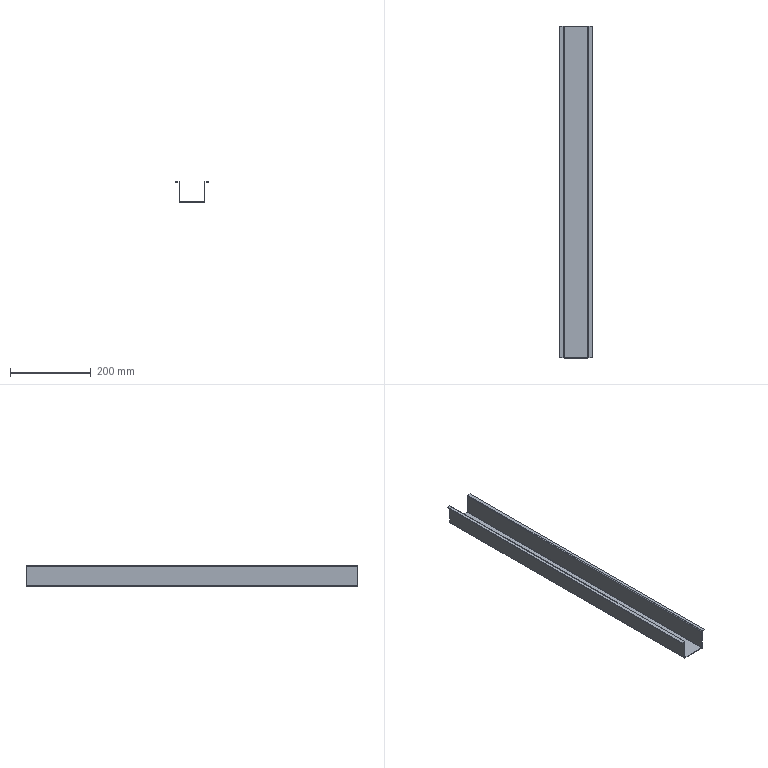Part | SolidWorks | features BaseBody 1 | 1 solid | 38 faces | box 80 x 820 x 51.5 mm | volume 218760 mm3 | plane 30 | cylinder 8 | commonest cylinder face diameters 1 x4 4 x4
STEP:
#1=CARTESIAN_POINT('',(40.,-410.,48.5));
#2=VERTEX_POINT('',#1);
#3=CARTESIAN_POINT('',(40.,410.,48.5));
#4=VERTEX_POINT('',#3);
#5=CARTESIAN_POINT('',(40.,410.,48.5));
#6=DIRECTION('',(0.,1.,0.));
#7=VECTOR('',#6,1000.);
#8=LINE('',#5,#7);
#9=EDGE_CURVE('',#2,#4,#8,.T.);
#10=ORIENTED_EDGE('',*,*,#9,.T.);
#11=CARTESIAN_POINT('',(40.,410.,50.));
#12=VERTEX_POINT('',#11);
#13=CARTESIAN_POINT('',(40.,410.,50.));
#14=DIRECTION('',(0.,0.,-1.));
#15=VECTOR('',#14,1000.);
#16=LINE('',#13,#15);
#17=EDGE_CURVE('',#12,#4,#16,.T.);
#18=ORIENTED_EDGE('',*,*,#17,.F.);
#19=CARTESIAN_POINT('',(40.,-410.,50.));
#20=VERTEX_POINT('',#19);
#21=CARTESIAN_POINT('',(40.,410.,50.));
#22=DIRECTION('',(0.,1.,0.));
#23=VECTOR('',#22,1000.);
#24=LINE('',#21,#23);
#25=EDGE_CURVE('',#20,#12,#24,.T.);
#26=ORIENTED_EDGE('',*,*,#25,.F.);
#27=CARTESIAN_POINT('',(40.,-410.,50.));
#28=DIRECTION('',(0.,0.,-1.));
#29=VECTOR('',#28,1000.);
#30=LINE('',#27,#29);
#31=EDGE_CURVE('',#20,#2,#30,.T.);
#32=ORIENTED_EDGE('',*,*,#31,.T.);
#33=EDGE_LOOP('',(#10,#18,#26,#32));
#34=FACE_OUTER_BOUND('',#33,.T.);
#35=CARTESIAN_POINT('',(40.,410.,50.));
#36=DIRECTION('',(-1.,0.,0.));
#37=DIRECTION('',(0.,1.,0.));
#38=AXIS2_PLACEMENT_3D('',#35,#36,#37);
#39=PLANE('',#38);
#40=ADVANCED_FACE('',(#34),#39,.F.);
#41=CARTESIAN_POINT('',(32.,-410.,48.5));
#42=VERTEX_POINT('',#41);
#43=CARTESIAN_POINT('',(40.,-410.,48.5));
#44=DIRECTION('',(1.,0.,0.));
#45=VECTOR('',#44,1000.);
#46=LINE('',#43,#45);
#47=EDGE_CURVE('',#42,#2,#46,.T.);
#48=ORIENTED_EDGE('',*,*,#47,.F.);
#49=CARTESIAN_POINT('',(32.,410.,48.5));
#50=VERTEX_POINT('',#49);
#51=CARTESIAN_POINT('',(32.,410.,48.5));
#52=DIRECTION('',(0.,-1.,0.));
#53=VECTOR('',#52,1000.);
#54=LINE('',#51,#53);
#55=EDGE_CURVE('',#50,#42,#54,.T.);
#56=ORIENTED_EDGE('',*,*,#55,.F.);
#57=CARTESIAN_POINT('',(31.5,410.,48.5));
#58=DIRECTION('',(-1.,0.,0.));
#59=VECTOR('',#58,1000.);
#60=LINE('',#57,#59);
#61=EDGE_CURVE('',#4,#50,#60,.T.);
#62=ORIENTED_EDGE('',*,*,#61,.F.);
#63=ORIENTED_EDGE('',*,*,#9,.F.);
#64=EDGE_LOOP('',(#48,#56,#62,#63));
#65=FACE_OUTER_BOUND('',#64,.T.);
#66=CARTESIAN_POINT('',(0.,0.,48.5));
#67=DIRECTION('',(0.,0.,-1.));
#68=DIRECTION('',(0.,-1.,0.));
#69=AXIS2_PLACEMENT_3D('',#66,#67,#68);
#70=PLANE('',#69);
#71=ADVANCED_FACE('',(#65),#70,.T.);
#72=CARTESIAN_POINT('',(32.,-410.,50.));
#73=VERTEX_POINT('',#72);
#74=CARTESIAN_POINT('',(32.,410.,50.));
#75=VERTEX_POINT('',#74);
#76=CARTESIAN_POINT('',(32.,0.,50.));
#77=DIRECTION('',(0.,1.,0.));
#78=VECTOR('',#77,1000.);
#79=LINE('',#76,#78);
#80=EDGE_CURVE('',#73,#75,#79,.T.);
#81=ORIENTED_EDGE('',*,*,#80,.F.);
#82=CARTESIAN_POINT('',(40.,-410.,50.));
#83=DIRECTION('',(1.,0.,0.));
#84=VECTOR('',#83,1000.);
#85=LINE('',#82,#84);
#86=EDGE_CURVE('',#73,#20,#85,.T.);
#87=ORIENTED_EDGE('',*,*,#86,.T.);
#88=ORIENTED_EDGE('',*,*,#25,.T.);
#89=CARTESIAN_POINT('',(31.5,410.,50.));
#90=DIRECTION('',(-1.,0.,0.));
#91=VECTOR('',#90,1000.);
#92=LINE('',#89,#91);
#93=EDGE_CURVE('',#12,#75,#92,.T.);
#94=ORIENTED_EDGE('',*,*,#93,.T.);
#95=EDGE_LOOP('',(#81,#87,#88,#94));
#96=FACE_OUTER_BOUND('',#95,.T.);
#97=CARTESIAN_POINT('',(0.,0.,50.));
#98=DIRECTION('',(0.,0.,-1.));
#99=DIRECTION('',(0.,-1.,0.));
#100=AXIS2_PLACEMENT_3D('',#97,#98,#99);
#101=PLANE('',#100);
#102=ADVANCED_FACE('',(#96),#101,.F.);
#103=CARTESIAN_POINT('',(32.,-410.,48.5));
#104=DIRECTION('',(0.,0.,1.));
#105=VECTOR('',#104,1000.);
#106=LINE('',#103,#105);
#107=EDGE_CURVE('',#42,#73,#106,.T.);
#108=ORIENTED_EDGE('',*,*,#107,.F.);
#109=ORIENTED_EDGE('',*,*,#47,.T.);
#110=ORIENTED_EDGE('',*,*,#31,.F.);
#111=ORIENTED_EDGE('',*,*,#86,.F.);
#112=EDGE_LOOP('',(#108,#109,#110,#111));
#113=FACE_OUTER_BOUND('',#112,.T.);
#114=CARTESIAN_POINT('',(40.,-410.,50.));
#115=DIRECTION('',(0.,1.,0.));
#116=DIRECTION('',(0.,0.,-1.));
#117=AXIS2_PLACEMENT_3D('',#114,#115,#116);
#118=PLANE('',#117);
#119=ADVANCED_FACE('',(#113),#118,.F.);
#120=CARTESIAN_POINT('',(32.,410.,48.5));
#121=DIRECTION('',(0.,0.,1.));
#122=VECTOR('',#121,1000.);
#123=LINE('',#120,#122);
#124=EDGE_CURVE('',#50,#75,#123,.T.);
#125=ORIENTED_EDGE('',*,*,#124,.T.);
#126=ORIENTED_EDGE('',*,*,#93,.F.);
#127=ORIENTED_EDGE('',*,*,#17,.T.);
#128=ORIENTED_EDGE('',*,*,#61,.T.);
#129=EDGE_LOOP('',(#125,#126,#127,#128));
#130=FACE_OUTER_BOUND('',#129,.T.);
#131=CARTESIAN_POINT('',(31.5,410.,50.));
#132=DIRECTION('',(0.,-1.,0.));
#133=DIRECTION('',(-1.,0.,0.));
#134=AXIS2_PLACEMENT_3D('',#131,#132,#133);
#135=PLANE('',#134);
#136=ADVANCED_FACE('',(#130),#135,.F.);
#137=CARTESIAN_POINT('',(31.5,-410.,48.));
#138=VERTEX_POINT('',#137);
#139=CARTESIAN_POINT('',(31.5,410.,48.));
#140=VERTEX_POINT('',#139);
#141=CARTESIAN_POINT('',(31.5,-410.,48.));
#142=DIRECTION('',(0.,1.,0.));
#143=VECTOR('',#142,1000.);
#144=LINE('',#141,#143);
#145=EDGE_CURVE('',#138,#140,#144,.T.);
#146=ORIENTED_EDGE('',*,*,#145,.T.);
#147=CARTESIAN_POINT('',(32.,410.,48.));
#148=DIRECTION('',(0.,1.,0.));
#149=DIRECTION('',(0.,0.,-1.));
#150=AXIS2_PLACEMENT_3D('',#147,#148,#149);
#151=CIRCLE('',#150,0.5);
#152=EDGE_CURVE('',#140,#50,#151,.T.);
#153=ORIENTED_EDGE('',*,*,#152,.T.);
#154=ORIENTED_EDGE('',*,*,#55,.T.);
#155=CARTESIAN_POINT('',(32.,-410.,48.));
#156=DIRECTION('',(0.,-1.,0.));
#157=DIRECTION('',(0.,0.,-1.));
#158=AXIS2_PLACEMENT_3D('',#155,#156,#157);
#159=CIRCLE('',#158,0.5);
#160=EDGE_CURVE('',#42,#138,#159,.T.);
#161=ORIENTED_EDGE('',*,*,#160,.T.);
#162=EDGE_LOOP('',(#146,#153,#154,#161));
#163=FACE_OUTER_BOUND('',#162,.T.);
#164=CARTESIAN_POINT('',(32.,-410.,48.));
#165=DIRECTION('',(0.,-1.,0.));
#166=DIRECTION('',(0.,0.,1.));
#167=AXIS2_PLACEMENT_3D('',#164,#165,#166);
#168=CYLINDRICAL_SURFACE('',#167,0.5);
#169=ADVANCED_FACE('',(#163),#168,.F.);
#170=CARTESIAN_POINT('',(30.,-410.,48.));
#171=VERTEX_POINT('',#170);
#172=CARTESIAN_POINT('',(30.,410.,48.));
#173=VERTEX_POINT('',#172);
#174=CARTESIAN_POINT('',(30.,-410.,48.));
#175=DIRECTION('',(0.,1.,0.));
#176=VECTOR('',#175,1000.);
#177=LINE('',#174,#176);
#178=EDGE_CURVE('',#171,#173,#177,.T.);
#179=ORIENTED_EDGE('',*,*,#178,.F.);
#180=CARTESIAN_POINT('',(32.,-410.,48.));
#181=DIRECTION('',(0.,-1.,0.));
#182=DIRECTION('',(0.,0.,-1.));
#183=AXIS2_PLACEMENT_3D('',#180,#181,#182);
#184=CIRCLE('',#183,2.);
#185=EDGE_CURVE('',#73,#171,#184,.T.);
#186=ORIENTED_EDGE('',*,*,#185,.F.);
#187=ORIENTED_EDGE('',*,*,#80,.T.);
#188=CARTESIAN_POINT('',(32.,410.,48.));
#189=DIRECTION('',(0.,1.,0.));
#190=DIRECTION('',(0.,0.,-1.));
#191=AXIS2_PLACEMENT_3D('',#188,#189,#190);
#192=CIRCLE('',#191,2.);
#193=EDGE_CURVE('',#173,#75,#192,.T.);
#194=ORIENTED_EDGE('',*,*,#193,.F.);
#195=EDGE_LOOP('',(#179,#186,#187,#194));
#196=FACE_OUTER_BOUND('',#195,.T.);
#197=CARTESIAN_POINT('',(32.,-410.,48.));
#198=DIRECTION('',(0.,-1.,0.));
#199=DIRECTION('',(0.,0.,1.));
#200=AXIS2_PLACEMENT_3D('',#197,#198,#199);
#201=CYLINDRICAL_SURFACE('',#200,2.);
#202=ADVANCED_FACE('',(#196),#201,.T.);
#203=ORIENTED_EDGE('',*,*,#160,.F.);
#204=ORIENTED_EDGE('',*,*,#107,.T.);
#205=ORIENTED_EDGE('',*,*,#185,.T.);
#206=CARTESIAN_POINT('',(31.5,-410.,48.));
#207=DIRECTION('',(-1.,0.,0.));
#208=VECTOR('',#207,1000.);
#209=LINE('',#206,#208);
#210=EDGE_CURVE('',#138,#171,#209,.T.);
#211=ORIENTED_EDGE('',*,*,#210,.F.);
#212=EDGE_LOOP('',(#203,#204,#205,#211));
#213=FACE_OUTER_BOUND('',#212,.T.);
#214=CARTESIAN_POINT('',(32.,-410.,48.));
#215=DIRECTION('',(0.,1.,0.));
#216=DIRECTION('',(1.,0.,0.));
#217=AXIS2_PLACEMENT_3D('',#214,#215,#216);
#218=PLANE('',#217);
#219=ADVANCED_FACE('',(#213),#218,.F.);
#220=ORIENTED_EDGE('',*,*,#124,.F.);
#221=ORIENTED_EDGE('',*,*,#152,.F.);
#222=CARTESIAN_POINT('',(31.5,410.,48.));
#223=DIRECTION('',(-1.,0.,0.));
#224=VECTOR('',#223,1000.);
#225=LINE('',#222,#224);
#226=EDGE_CURVE('',#140,#173,#225,.T.);
#227=ORIENTED_EDGE('',*,*,#226,.T.);
#228=ORIENTED_EDGE('',*,*,#193,.T.);
#229=EDGE_LOOP('',(#220,#221,#227,#228));
#230=FACE_OUTER_BOUND('',#229,.T.);
#231=CARTESIAN_POINT('',(32.,410.,48.));
#232=DIRECTION('',(0.,1.,0.));
#233=DIRECTION('',(1.,0.,0.));
#234=AXIS2_PLACEMENT_3D('',#231,#232,#233);
#235=PLANE('',#234);
#236=ADVANCED_FACE('',(#230),#235,.T.);
#237=CARTESIAN_POINT('',(-40.,410.,48.5));
#238=VERTEX_POINT('',#237);
#239=CARTESIAN_POINT('',(-40.,-410.,48.5));
#240=VERTEX_POINT('',#239);
#241=CARTESIAN_POINT('',(-40.,-410.,48.5));
#242=DIRECTION('',(0.,-1.,0.));
#243=VECTOR('',#242,1000.);
#244=LINE('',#241,#243);
#245=EDGE_CURVE('',#238,#240,#244,.T.);
#246=ORIENTED_EDGE('',*,*,#245,.T.);
#247=CARTESIAN_POINT('',(-40.,-410.,50.));
#248=VERTEX_POINT('',#247);
#249=CARTESIAN_POINT('',(-40.,-410.,50.));
#250=DIRECTION('',(0.,0.,-1.));
#251=VECTOR('',#250,1000.);
#252=LINE('',#249,#251);
#253=EDGE_CURVE('',#248,#240,#252,.T.);
#254=ORIENTED_EDGE('',*,*,#253,.F.);
#255=CARTESIAN_POINT('',(-40.,410.,50.));
#256=VERTEX_POINT('',#255);
#257=CARTESIAN_POINT('',(-40.,-410.,50.));
#258=DIRECTION('',(0.,-1.,0.));
#259=VECTOR('',#258,1000.);
#260=LINE('',#257,#259);
#261=EDGE_CURVE('',#256,#248,#260,.T.);
#262=ORIENTED_EDGE('',*,*,#261,.F.);
#263=CARTESIAN_POINT('',(-40.,410.,50.));
#264=DIRECTION('',(0.,0.,-1.));
#265=VECTOR('',#264,1000.);
#266=LINE('',#263,#265);
#267=EDGE_CURVE('',#256,#238,#266,.T.);
#268=ORIENTED_EDGE('',*,*,#267,.T.);
#269=EDGE_LOOP('',(#246,#254,#262,#268));
#270=FACE_OUTER_BOUND('',#269,.T.);
#271=CARTESIAN_POINT('',(-40.,-410.,50.));
#272=DIRECTION('',(1.,0.,0.));
#273=DIRECTION('',(0.,1.,0.));
#274=AXIS2_PLACEMENT_3D('',#271,#272,#273);
#275=PLANE('',#274);
#276=ADVANCED_FACE('',(#270),#275,.F.);
#277=CARTESIAN_POINT('',(-32.,410.,48.5));
#278=VERTEX_POINT('',#277);
#279=CARTESIAN_POINT('',(-40.,410.,48.5));
#280=DIRECTION('',(-1.,0.,0.));
#281=VECTOR('',#280,1000.);
#282=LINE('',#279,#281);
#283=EDGE_CURVE('',#278,#238,#282,.T.);
#284=ORIENTED_EDGE('',*,*,#283,.F.);
#285=CARTESIAN_POINT('',(-32.,-410.,48.5));
#286=VERTEX_POINT('',#285);
#287=CARTESIAN_POINT('',(-32.,-410.,48.5));
#288=DIRECTION('',(0.,1.,0.));
#289=VECTOR('',#288,1000.);
#290=LINE('',#287,#289);
#291=EDGE_CURVE('',#286,#278,#290,.T.);
#292=ORIENTED_EDGE('',*,*,#291,.F.);
#293=CARTESIAN_POINT('',(-31.5,-410.,48.5));
#294=DIRECTION('',(1.,0.,0.));
#295=VECTOR('',#294,1000.);
#296=LINE('',#293,#295);
#297=EDGE_CURVE('',#240,#286,#296,.T.);
#298=ORIENTED_EDGE('',*,*,#297,.F.);
#299=ORIENTED_EDGE('',*,*,#245,.F.);
#300=EDGE_LOOP('',(#284,#292,#298,#299));
#301=FACE_OUTER_BOUND('',#300,.T.);
#302=CARTESIAN_POINT('',(0.,0.,48.5));
#303=DIRECTION('',(0.,0.,-1.));
#304=DIRECTION('',(0.,-1.,0.));
#305=AXIS2_PLACEMENT_3D('',#302,#303,#304);
#306=PLANE('',#305);
#307=ADVANCED_FACE('',(#301),#306,.T.);
#308=CARTESIAN_POINT('',(-32.,410.,50.));
#309=VERTEX_POINT('',#308);
#310=CARTESIAN_POINT('',(-32.,-410.,50.));
#311=VERTEX_POINT('',#310);
#312=CARTESIAN_POINT('',(-32.,0.,50.));
#313=DIRECTION('',(0.,-1.,0.));
#314=VECTOR('',#313,1000.);
#315=LINE('',#312,#314);
#316=EDGE_CURVE('',#309,#311,#315,.T.);
#317=ORIENTED_EDGE('',*,*,#316,.F.);
#318=CARTESIAN_POINT('',(-40.,410.,50.));
#319=DIRECTION('',(-1.,0.,0.));
#320=VECTOR('',#319,1000.);
#321=LINE('',#318,#320);
#322=EDGE_CURVE('',#309,#256,#321,.T.);
#323=ORIENTED_EDGE('',*,*,#322,.T.);
#324=ORIENTED_EDGE('',*,*,#261,.T.);
#325=CARTESIAN_POINT('',(-31.5,-410.,50.));
#326=DIRECTION('',(1.,0.,0.));
#327=VECTOR('',#326,1000.);
#328=LINE('',#325,#327);
#329=EDGE_CURVE('',#248,#311,#328,.T.);
#330=ORIENTED_EDGE('',*,*,#329,.T.);
#331=EDGE_LOOP('',(#317,#323,#324,#330));
#332=FACE_OUTER_BOUND('',#331,.T.);
#333=CARTESIAN_POINT('',(0.,0.,50.));
#334=DIRECTION('',(0.,0.,-1.));
#335=DIRECTION('',(0.,-1.,0.));
#336=AXIS2_PLACEMENT_3D('',#333,#334,#335);
#337=PLANE('',#336);
#338=ADVANCED_FACE('',(#332),#337,.F.);
#339=CARTESIAN_POINT('',(-32.,410.,48.5));
#340=DIRECTION('',(0.,0.,1.));
#341=VECTOR('',#340,1000.);
#342=LINE('',#339,#341);
#343=EDGE_CURVE('',#278,#309,#342,.T.);
#344=ORIENTED_EDGE('',*,*,#343,.F.);
#345=ORIENTED_EDGE('',*,*,#283,.T.);
#346=ORIENTED_EDGE('',*,*,#267,.F.);
#347=ORIENTED_EDGE('',*,*,#322,.F.);
#348=EDGE_LOOP('',(#344,#345,#346,#347));
#349=FACE_OUTER_BOUND('',#348,.T.);
#350=CARTESIAN_POINT('',(-40.,410.,50.));
#351=DIRECTION('',(0.,-1.,0.));
#352=DIRECTION('',(0.,0.,-1.));
#353=AXIS2_PLACEMENT_3D('',#350,#351,#352);
#354=PLANE('',#353);
#355=ADVANCED_FACE('',(#349),#354,.F.);
#356=CARTESIAN_POINT('',(-32.,-410.,48.5));
#357=DIRECTION('',(0.,0.,1.));
#358=VECTOR('',#357,1000.);
#359=LINE('',#356,#358);
#360=EDGE_CURVE('',#286,#311,#359,.T.);
#361=ORIENTED_EDGE('',*,*,#360,.T.);
#362=ORIENTED_EDGE('',*,*,#329,.F.);
#363=ORIENTED_EDGE('',*,*,#253,.T.);
#364=ORIENTED_EDGE('',*,*,#297,.T.);
#365=EDGE_LOOP('',(#361,#362,#363,#364));
#366=FACE_OUTER_BOUND('',#365,.T.);
#367=CARTESIAN_POINT('',(-31.5,-410.,50.));
#368=DIRECTION('',(0.,1.,0.));
#369=DIRECTION('',(0.,0.,-1.));
#370=AXIS2_PLACEMENT_3D('',#367,#368,#369);
#371=PLANE('',#370);
#372=ADVANCED_FACE('',(#366),#371,.F.);
#373=CARTESIAN_POINT('',(-31.5,410.,48.));
#374=VERTEX_POINT('',#373);
#375=CARTESIAN_POINT('',(-31.5,-410.,48.));
#376=VERTEX_POINT('',#375);
#377=CARTESIAN_POINT('',(-31.5,410.,48.));
#378=DIRECTION('',(0.,-1.,0.));
#379=VECTOR('',#378,1000.);
#380=LINE('',#377,#379);
#381=EDGE_CURVE('',#374,#376,#380,.T.);
#382=ORIENTED_EDGE('',*,*,#381,.T.);
#383=CARTESIAN_POINT('',(-32.,-410.,48.));
#384=DIRECTION('',(0.,-1.,0.));
#385=DIRECTION('',(0.,0.,1.));
#386=AXIS2_PLACEMENT_3D('',#383,#384,#385);
#387=CIRCLE('',#386,0.5);
#388=EDGE_CURVE('',#376,#286,#387,.T.);
#389=ORIENTED_EDGE('',*,*,#388,.T.);
#390=ORIENTED_EDGE('',*,*,#291,.T.);
#391=CARTESIAN_POINT('',(-32.,410.,48.));
#392=DIRECTION('',(0.,1.,0.));
#393=DIRECTION('',(0.,0.,1.));
#394=AXIS2_PLACEMENT_3D('',#391,#392,#393);
#395=CIRCLE('',#394,0.5);
#396=EDGE_CURVE('',#278,#374,#395,.T.);
#397=ORIENTED_EDGE('',*,*,#396,.T.);
#398=EDGE_LOOP('',(#382,#389,#390,#397));
#399=FACE_OUTER_BOUND('',#398,.T.);
#400=CARTESIAN_POINT('',(-32.,410.,48.));
#401=DIRECTION('',(0.,1.,0.));
#402=DIRECTION('',(0.,0.,1.));
#403=AXIS2_PLACEMENT_3D('',#400,#401,#402);
#404=CYLINDRICAL_SURFACE('',#403,0.5);
#405=ADVANCED_FACE('',(#399),#404,.F.);
#406=CARTESIAN_POINT('',(-30.,410.,48.));
#407=VERTEX_POINT('',#406);
#408=CARTESIAN_POINT('',(-30.,-410.,48.));
#409=VERTEX_POINT('',#408);
#410=CARTESIAN_POINT('',(-30.,410.,48.));
#411=DIRECTION('',(0.,-1.,0.));
#412=VECTOR('',#411,1000.);
#413=LINE('',#410,#412);
#414=EDGE_CURVE('',#407,#409,#413,.T.);
#415=ORIENTED_EDGE('',*,*,#414,.F.);
#416=CARTESIAN_POINT('',(-32.,410.,48.));
#417=DIRECTION('',(0.,1.,0.));
#418=DIRECTION('',(0.,0.,1.));
#419=AXIS2_PLACEMENT_3D('',#416,#417,#418);
#420=CIRCLE('',#419,2.);
#421=EDGE_CURVE('',#309,#407,#420,.T.);
#422=ORIENTED_EDGE('',*,*,#421,.F.);
#423=ORIENTED_EDGE('',*,*,#316,.T.);
#424=CARTESIAN_POINT('',(-32.,-410.,48.));
#425=DIRECTION('',(0.,-1.,0.));
#426=DIRECTION('',(0.,0.,1.));
#427=AXIS2_PLACEMENT_3D('',#424,#425,#426);
#428=CIRCLE('',#427,2.);
#429=EDGE_CURVE('',#409,#311,#428,.T.);
#430=ORIENTED_EDGE('',*,*,#429,.F.);
#431=EDGE_LOOP('',(#415,#422,#423,#430));
#432=FACE_OUTER_BOUND('',#431,.T.);
#433=CARTESIAN_POINT('',(-32.,410.,48.));
#434=DIRECTION('',(0.,1.,0.));
#435=DIRECTION('',(0.,0.,1.));
#436=AXIS2_PLACEMENT_3D('',#433,#434,#435);
#437=CYLINDRICAL_SURFACE('',#436,2.);
#438=ADVANCED_FACE('',(#432),#437,.T.);
#439=ORIENTED_EDGE('',*,*,#396,.F.);
#440=ORIENTED_EDGE('',*,*,#343,.T.);
#441=ORIENTED_EDGE('',*,*,#421,.T.);
#442=CARTESIAN_POINT('',(-31.5,410.,48.));
#443=DIRECTION('',(1.,0.,0.));
#444=VECTOR('',#443,1000.);
#445=LINE('',#442,#444);
#446=EDGE_CURVE('',#374,#407,#445,.T.);
#447=ORIENTED_EDGE('',*,*,#446,.F.);
#448=EDGE_LOOP('',(#439,#440,#441,#447));
#449=FACE_OUTER_BOUND('',#448,.T.);
#450=CARTESIAN_POINT('',(-32.,410.,48.));
#451=DIRECTION('',(0.,-1.,0.));
#452=DIRECTION('',(0.,0.,-1.));
#453=AXIS2_PLACEMENT_3D('',#450,#451,#452);
#454=PLANE('',#453);
#455=ADVANCED_FACE('',(#449),#454,.F.);
#456=ORIENTED_EDGE('',*,*,#360,.F.);
#457=ORIENTED_EDGE('',*,*,#388,.F.);
#458=CARTESIAN_POINT('',(-31.5,-410.,48.));
#459=DIRECTION('',(1.,0.,0.));
#460=VECTOR('',#459,1000.);
#461=LINE('',#458,#460);
#462=EDGE_CURVE('',#376,#409,#461,.T.);
#463=ORIENTED_EDGE('',*,*,#462,.T.);
#464=ORIENTED_EDGE('',*,*,#429,.T.);
#465=EDGE_LOOP('',(#456,#457,#463,#464));
#466=FACE_OUTER_BOUND('',#465,.T.);
#467=CARTESIAN_POINT('',(-32.,-410.,48.));
#468=DIRECTION('',(0.,-1.,0.));
#469=DIRECTION('',(0.,0.,-1.));
#470=AXIS2_PLACEMENT_3D('',#467,#468,#469);
#471=PLANE('',#470);
#472=ADVANCED_FACE('',(#466),#471,.T.);
#473=CARTESIAN_POINT('',(29.5,410.,0.));
#474=VERTEX_POINT('',#473);
#475=CARTESIAN_POINT('',(29.5,-410.,0.));
#476=VERTEX_POINT('',#475);
#477=CARTESIAN_POINT('',(29.5,410.,0.));
#478=DIRECTION('',(0.,-1.,0.));
#479=VECTOR('',#478,1000.);
#480=LINE('',#477,#479);
#481=EDGE_CURVE('',#474,#476,#480,.T.);
#482=ORIENTED_EDGE('',*,*,#481,.T.);
#483=CARTESIAN_POINT('',(30.,-410.,0.5));
#484=VERTEX_POINT('',#483);
#485=CARTESIAN_POINT('',(29.5,-410.,0.5));
#486=DIRECTION('',(0.,-1.,0.));
#487=DIRECTION('',(0.,0.,1.));
#488=AXIS2_PLACEMENT_3D('',#485,#486,#487);
#489=CIRCLE('',#488,0.5);
#490=EDGE_CURVE('',#476,#484,#489,.T.);
#491=ORIENTED_EDGE('',*,*,#490,.T.);
#492=CARTESIAN_POINT('',(30.,410.,0.5));
#493=VERTEX_POINT('',#492);
#494=CARTESIAN_POINT('',(30.,-410.,0.5));
#495=DIRECTION('',(0.,1.,0.));
#496=VECTOR('',#495,1000.);
#497=LINE('',#494,#496);
#498=EDGE_CURVE('',#484,#493,#497,.T.);
#499=ORIENTED_EDGE('',*,*,#498,.T.);
#500=CARTESIAN_POINT('',(29.5,410.,0.5));
#501=DIRECTION('',(0.,1.,0.));
#502=DIRECTION('',(0.,0.,1.));
#503=AXIS2_PLACEMENT_3D('',#500,#501,#502);
#504=CIRCLE('',#503,0.5);
#505=EDGE_CURVE('',#493,#474,#504,.T.);
#506=ORIENTED_EDGE('',*,*,#505,.T.);
#507=EDGE_LOOP('',(#482,#491,#499,#506));
#508=FACE_OUTER_BOUND('',#507,.T.);
#509=CARTESIAN_POINT('',(29.5,410.,0.5));
#510=DIRECTION('',(0.,1.,0.));
#511=DIRECTION('',(1.,0.,0.));
#512=AXIS2_PLACEMENT_3D('',#509,#510,#511);
#513=CYLINDRICAL_SURFACE('',#512,0.5);
#514=ADVANCED_FACE('',(#508),#513,.F.);
#515=CARTESIAN_POINT('',(29.5,410.,-1.5));
#516=VERTEX_POINT('',#515);
#517=CARTESIAN_POINT('',(29.5,-410.,-1.5));
#518=VERTEX_POINT('',#517);
#519=CARTESIAN_POINT('',(29.5,410.,-1.5));
#520=DIRECTION('',(0.,-1.,0.));
#521=VECTOR('',#520,1000.);
#522=LINE('',#519,#521);
#523=EDGE_CURVE('',#516,#518,#522,.T.);
#524=ORIENTED_EDGE('',*,*,#523,.F.);
#525=CARTESIAN_POINT('',(31.5,410.,0.5));
#526=VERTEX_POINT('',#525);
#527=CARTESIAN_POINT('',(29.5,410.,0.5));
#528=DIRECTION('',(0.,1.,0.));
#529=DIRECTION('',(0.,0.,1.));
#530=AXIS2_PLACEMENT_3D('',#527,#528,#529);
#531=CIRCLE('',#530,2.);
#532=EDGE_CURVE('',#526,#516,#531,.T.);
#533=ORIENTED_EDGE('',*,*,#532,.F.);
#534=CARTESIAN_POINT('',(31.5,-410.,0.5));
#535=VERTEX_POINT('',#534);
#536=CARTESIAN_POINT('',(31.5,0.,0.5));
#537=DIRECTION('',(0.,-1.,0.));
#538=VECTOR('',#537,1000.);
#539=LINE('',#536,#538);
#540=EDGE_CURVE('',#526,#535,#539,.T.);
#541=ORIENTED_EDGE('',*,*,#540,.T.);
#542=CARTESIAN_POINT('',(29.5,-410.,0.5));
#543=DIRECTION('',(0.,-1.,0.));
#544=DIRECTION('',(0.,0.,1.));
#545=AXIS2_PLACEMENT_3D('',#542,#543,#544);
#546=CIRCLE('',#545,2.);
#547=EDGE_CURVE('',#518,#535,#546,.T.);
#548=ORIENTED_EDGE('',*,*,#547,.F.);
#549=EDGE_LOOP('',(#524,#533,#541,#548));
#550=FACE_OUTER_BOUND('',#549,.T.);
#551=CARTESIAN_POINT('',(29.5,410.,0.5));
#552=DIRECTION('',(0.,1.,0.));
#553=DIRECTION('',(1.,0.,0.));
#554=AXIS2_PLACEMENT_3D('',#551,#552,#553);
#555=CYLINDRICAL_SURFACE('',#554,2.);
#556=ADVANCED_FACE('',(#550),#555,.T.);
#557=ORIENTED_EDGE('',*,*,#505,.F.);
#558=CARTESIAN_POINT('',(30.,410.,0.5));
#559=DIRECTION('',(1.,0.,0.));
#560=VECTOR('',#559,1000.);
#561=LINE('',#558,#560);
#562=EDGE_CURVE('',#493,#526,#561,.T.);
#563=ORIENTED_EDGE('',*,*,#562,.T.);
#564=ORIENTED_EDGE('',*,*,#532,.T.);
#565=CARTESIAN_POINT('',(29.5,410.,0.));
#566=DIRECTION('',(0.,0.,-1.));
#567=VECTOR('',#566,1000.);
#568=LINE('',#565,#567);
#569=EDGE_CURVE('',#474,#516,#568,.T.);
#570=ORIENTED_EDGE('',*,*,#569,.F.);
#571=EDGE_LOOP('',(#557,#563,#564,#570));
#572=FACE_OUTER_BOUND('',#571,.T.);
#573=CARTESIAN_POINT('',(29.5,410.,0.5));
#574=DIRECTION('',(0.,-1.,0.));
#575=DIRECTION('',(0.,0.,-1.));
#576=AXIS2_PLACEMENT_3D('',#573,#574,#575);
#577=PLANE('',#576);
#578=ADVANCED_FACE('',(#572),#577,.F.);
#579=CARTESIAN_POINT('',(30.,-410.,0.5));
#580=DIRECTION('',(1.,0.,0.));
#581=VECTOR('',#580,1000.);
#582=LINE('',#579,#581);
#583=EDGE_CURVE('',#484,#535,#582,.T.);
#584=ORIENTED_EDGE('',*,*,#583,.F.);
#585=ORIENTED_EDGE('',*,*,#490,.F.);
#586=CARTESIAN_POINT('',(29.5,-410.,0.));
#587=DIRECTION('',(0.,0.,-1.));
#588=VECTOR('',#587,1000.);
#589=LINE('',#586,#588);
#590=EDGE_CURVE('',#476,#518,#589,.T.);
#591=ORIENTED_EDGE('',*,*,#590,.T.);
#592=ORIENTED_EDGE('',*,*,#547,.T.);
#593=EDGE_LOOP('',(#584,#585,#591,#592));
#594=FACE_OUTER_BOUND('',#593,.T.);
#595=CARTESIAN_POINT('',(29.5,-410.,0.5));
#596=DIRECTION('',(0.,-1.,0.));
#597=DIRECTION('',(0.,0.,-1.));
#598=AXIS2_PLACEMENT_3D('',#595,#596,#597);
#599=PLANE('',#598);
#600=ADVANCED_FACE('',(#594),#599,.T.);
#601=CARTESIAN_POINT('',(-29.5,-410.,0.));
#602=VERTEX_POINT('',#601);
#603=CARTESIAN_POINT('',(-29.5,410.,0.));
#604=VERTEX_POINT('',#603);
#605=CARTESIAN_POINT('',(-29.5,-410.,0.));
#606=DIRECTION('',(0.,1.,0.));
#607=VECTOR('',#606,1000.);
#608=LINE('',#605,#607);
#609=EDGE_CURVE('',#602,#604,#608,.T.);
#610=ORIENTED_EDGE('',*,*,#609,.T.);
#611=CARTESIAN_POINT('',(-30.,410.,0.5));
#612=VERTEX_POINT('',#611);
#613=CARTESIAN_POINT('',(-29.5,410.,0.5));
#614=DIRECTION('',(0.,1.,0.));
#615=DIRECTION('',(0.,0.,-1.));
#616=AXIS2_PLACEMENT_3D('',#613,#614,#615);
#617=CIRCLE('',#616,0.5);
#618=EDGE_CURVE('',#604,#612,#617,.T.);
#619=ORIENTED_EDGE('',*,*,#618,.T.);
#620=CARTESIAN_POINT('',(-30.,-410.,0.5));
#621=VERTEX_POINT('',#620);
#622=CARTESIAN_POINT('',(-30.,410.,0.5));
#623=DIRECTION('',(0.,-1.,0.));
#624=VECTOR('',#623,1000.);
#625=LINE('',#622,#624);
#626=EDGE_CURVE('',#612,#621,#625,.T.);
#627=ORIENTED_EDGE('',*,*,#626,.T.);
#628=CARTESIAN_POINT('',(-29.5,-410.,0.5));
#629=DIRECTION('',(0.,-1.,0.));
#630=DIRECTION('',(0.,0.,-1.));
#631=AXIS2_PLACEMENT_3D('',#628,#629,#630);
#632=CIRCLE('',#631,0.5);
#633=EDGE_CURVE('',#621,#602,#632,.T.);
#634=ORIENTED_EDGE('',*,*,#633,.T.);
#635=EDGE_LOOP('',(#610,#619,#627,#634));
#636=FACE_OUTER_BOUND('',#635,.T.);
#637=CARTESIAN_POINT('',(-29.5,-410.,0.5));
#638=DIRECTION('',(0.,-1.,0.));
#639=DIRECTION('',(-1.,0.,0.));
#640=AXIS2_PLACEMENT_3D('',#637,#638,#639);
#641=CYLINDRICAL_SURFACE('',#640,0.5);
#642=ADVANCED_FACE('',(#636),#641,.F.);
#643=CARTESIAN_POINT('',(-29.5,-410.,-1.5));
#644=VERTEX_POINT('',#643);
#645=CARTESIAN_POINT('',(-29.5,410.,-1.5));
#646=VERTEX_POINT('',#645);
#647=CARTESIAN_POINT('',(-29.5,-410.,-1.5));
#648=DIRECTION('',(0.,1.,0.));
#649=VECTOR('',#648,1000.);
#650=LINE('',#647,#649);
#651=EDGE_CURVE('',#644,#646,#650,.T.);
#652=ORIENTED_EDGE('',*,*,#651,.F.);
#653=CARTESIAN_POINT('',(-31.5,-410.,0.5));
#654=VERTEX_POINT('',#653);
#655=CARTESIAN_POINT('',(-29.5,-410.,0.5));
#656=DIRECTION('',(0.,-1.,0.));
#657=DIRECTION('',(0.,0.,-1.));
#658=AXIS2_PLACEMENT_3D('',#655,#656,#657);
#659=CIRCLE('',#658,2.);
#660=EDGE_CURVE('',#654,#644,#659,.T.);
#661=ORIENTED_EDGE('',*,*,#660,.F.);
#662=CARTESIAN_POINT('',(-31.5,410.,0.5));
#663=VERTEX_POINT('',#662);
#664=CARTESIAN_POINT('',(-31.5,0.,0.5));
#665=DIRECTION('',(0.,1.,0.));
#666=VECTOR('',#665,1000.);
#667=LINE('',#664,#666);
#668=EDGE_CURVE('',#654,#663,#667,.T.);
#669=ORIENTED_EDGE('',*,*,#668,.T.);
#670=CARTESIAN_POINT('',(-29.5,410.,0.5));
#671=DIRECTION('',(0.,1.,0.));
#672=DIRECTION('',(0.,0.,-1.));
#673=AXIS2_PLACEMENT_3D('',#670,#671,#672);
#674=CIRCLE('',#673,2.);
#675=EDGE_CURVE('',#646,#663,#674,.T.);
#676=ORIENTED_EDGE('',*,*,#675,.F.);
#677=EDGE_LOOP('',(#652,#661,#669,#676));
#678=FACE_OUTER_BOUND('',#677,.T.);
#679=CARTESIAN_POINT('',(-29.5,-410.,0.5));
#680=DIRECTION('',(0.,-1.,0.));
#681=DIRECTION('',(-1.,0.,0.));
#682=AXIS2_PLACEMENT_3D('',#679,#680,#681);
#683=CYLINDRICAL_SURFACE('',#682,2.);
#684=ADVANCED_FACE('',(#678),#683,.T.);
#685=ORIENTED_EDGE('',*,*,#633,.F.);
#686=CARTESIAN_POINT('',(-30.,-410.,0.5));
#687=DIRECTION('',(-1.,0.,0.));
#688=VECTOR('',#687,1000.);
#689=LINE('',#686,#688);
#690=EDGE_CURVE('',#621,#654,#689,.T.);
#691=ORIENTED_EDGE('',*,*,#690,.T.);
#692=ORIENTED_EDGE('',*,*,#660,.T.);
#693=CARTESIAN_POINT('',(-29.5,-410.,0.));
#694=DIRECTION('',(0.,0.,-1.));
#695=VECTOR('',#694,1000.);
#696=LINE('',#693,#695);
#697=EDGE_CURVE('',#602,#644,#696,.T.);
#698=ORIENTED_EDGE('',*,*,#697,.F.);
#699=EDGE_LOOP('',(#685,#691,#692,#698));
#700=FACE_OUTER_BOUND('',#699,.T.);
#701=CARTESIAN_POINT('',(-29.5,-410.,0.5));
#702=DIRECTION('',(0.,1.,0.));
#703=DIRECTION('',(1.,0.,0.));
#704=AXIS2_PLACEMENT_3D('',#701,#702,#703);
#705=PLANE('',#704);
#706=ADVANCED_FACE('',(#700),#705,.F.);
#707=CARTESIAN_POINT('',(-30.,410.,0.5));
#708=DIRECTION('',(-1.,0.,0.));
#709=VECTOR('',#708,1000.);
#710=LINE('',#707,#709);
#711=EDGE_CURVE('',#612,#663,#710,.T.);
#712=ORIENTED_EDGE('',*,*,#711,.F.);
#713=ORIENTED_EDGE('',*,*,#618,.F.);
#714=CARTESIAN_POINT('',(-29.5,410.,0.));
#715=DIRECTION('',(0.,0.,-1.));
#716=VECTOR('',#715,1000.);
#717=LINE('',#714,#716);
#718=EDGE_CURVE('',#604,#646,#717,.T.);
#719=ORIENTED_EDGE('',*,*,#718,.T.);
#720=ORIENTED_EDGE('',*,*,#675,.T.);
#721=EDGE_LOOP('',(#712,#713,#719,#720));
#722=FACE_OUTER_BOUND('',#721,.T.);
#723=CARTESIAN_POINT('',(-29.5,410.,0.5));
#724=DIRECTION('',(0.,1.,0.));
#725=DIRECTION('',(1.,0.,0.));
#726=AXIS2_PLACEMENT_3D('',#723,#724,#725);
#727=PLANE('',#726);
#728=ADVANCED_FACE('',(#722),#727,.T.);
#729=ORIENTED_EDGE('',*,*,#590,.F.);
#730=CARTESIAN_POINT('',(30.,-410.,0.));
#731=DIRECTION('',(1.,0.,0.));
#732=VECTOR('',#731,1000.);
#733=LINE('',#730,#732);
#734=EDGE_CURVE('',#602,#476,#733,.T.);
#735=ORIENTED_EDGE('',*,*,#734,.F.);
#736=ORIENTED_EDGE('',*,*,#697,.T.);
#737=CARTESIAN_POINT('',(30.,-410.,-1.5));
#738=DIRECTION('',(1.,0.,0.));
#739=VECTOR('',#738,1000.);
#740=LINE('',#737,#739);
#741=EDGE_CURVE('',#644,#518,#740,.T.);
#742=ORIENTED_EDGE('',*,*,#741,.T.);
#743=EDGE_LOOP('',(#729,#735,#736,#742));
#744=FACE_OUTER_BOUND('',#743,.T.);
#745=CARTESIAN_POINT('',(30.,-410.,-1.5));
#746=DIRECTION('',(0.,-1.,0.));
#747=DIRECTION('',(0.,0.,-1.));
#748=AXIS2_PLACEMENT_3D('',#745,#746,#747);
#749=PLANE('',#748);
#750=ADVANCED_FACE('',(#744),#749,.T.);
#751=CARTESIAN_POINT('',(30.,410.,0.));
#752=DIRECTION('',(-1.,0.,0.));
#753=VECTOR('',#752,1000.);
#754=LINE('',#751,#753);
#755=EDGE_CURVE('',#474,#604,#754,.T.);
#756=ORIENTED_EDGE('',*,*,#755,.F.);
#757=ORIENTED_EDGE('',*,*,#569,.T.);
#758=CARTESIAN_POINT('',(30.,410.,-1.5));
#759=DIRECTION('',(-1.,0.,0.));
#760=VECTOR('',#759,1000.);
#761=LINE('',#758,#760);
#762=EDGE_CURVE('',#516,#646,#761,.T.);
#763=ORIENTED_EDGE('',*,*,#762,.T.);
#764=ORIENTED_EDGE('',*,*,#718,.F.);
#765=EDGE_LOOP('',(#756,#757,#763,#764));
#766=FACE_OUTER_BOUND('',#765,.T.);
#767=CARTESIAN_POINT('',(30.,410.,-1.5));
#768=DIRECTION('',(0.,1.,0.));
#769=DIRECTION('',(1.,0.,0.));
#770=AXIS2_PLACEMENT_3D('',#767,#768,#769);
#771=PLANE('',#770);
#772=ADVANCED_FACE('',(#766),#771,.T.);
#773=ORIENTED_EDGE('',*,*,#481,.F.);
#774=ORIENTED_EDGE('',*,*,#755,.T.);
#775=ORIENTED_EDGE('',*,*,#609,.F.);
#776=ORIENTED_EDGE('',*,*,#734,.T.);
#777=EDGE_LOOP('',(#773,#774,#775,#776));
#778=FACE_OUTER_BOUND('',#777,.T.);
#779=CARTESIAN_POINT('',(0.,0.,0.));
#780=DIRECTION('',(0.,0.,-1.));
#781=DIRECTION('',(0.,-1.,0.));
#782=AXIS2_PLACEMENT_3D('',#779,#780,#781);
#783=PLANE('',#782);
#784=ADVANCED_FACE('',(#778),#783,.F.);
#785=ORIENTED_EDGE('',*,*,#762,.F.);
#786=ORIENTED_EDGE('',*,*,#523,.T.);
#787=ORIENTED_EDGE('',*,*,#741,.F.);
#788=ORIENTED_EDGE('',*,*,#651,.T.);
#789=EDGE_LOOP('',(#785,#786,#787,#788));
#790=FACE_OUTER_BOUND('',#789,.T.);
#791=CARTESIAN_POINT('',(0.,0.,-1.5));
#792=DIRECTION('',(0.,0.,-1.));
#793=DIRECTION('',(0.,-1.,0.));
#794=AXIS2_PLACEMENT_3D('',#791,#792,#793);
#795=PLANE('',#794);
#796=ADVANCED_FACE('',(#790),#795,.T.);
#797=CARTESIAN_POINT('',(-30.,410.,0.));
#798=DIRECTION('',(0.,0.,-1.));
#799=VECTOR('',#798,1000.);
#800=LINE('',#797,#799);
#801=EDGE_CURVE('',#407,#612,#800,.T.);
#802=ORIENTED_EDGE('',*,*,#801,.F.);
#803=ORIENTED_EDGE('',*,*,#414,.T.);
#804=CARTESIAN_POINT('',(-30.,-410.,48.5));
#805=DIRECTION('',(0.,0.,1.));
#806=VECTOR('',#805,1000.);
#807=LINE('',#804,#806);
#808=EDGE_CURVE('',#621,#409,#807,.T.);
#809=ORIENTED_EDGE('',*,*,#808,.F.);
#810=ORIENTED_EDGE('',*,*,#626,.F.);
#811=EDGE_LOOP('',(#802,#803,#809,#810));
#812=FACE_OUTER_BOUND('',#811,.T.);
#813=CARTESIAN_POINT('',(-30.,0.,0.));
#814=DIRECTION('',(1.,0.,0.));
#815=DIRECTION('',(0.,0.,1.));
#816=AXIS2_PLACEMENT_3D('',#813,#814,#815);
#817=PLANE('',#816);
#818=ADVANCED_FACE('',(#812),#817,.T.);
#819=ORIENTED_EDGE('',*,*,#381,.F.);
#820=CARTESIAN_POINT('',(-31.5,410.,0.));
#821=DIRECTION('',(0.,0.,-1.));
#822=VECTOR('',#821,1000.);
#823=LINE('',#820,#822);
#824=EDGE_CURVE('',#374,#663,#823,.T.);
#825=ORIENTED_EDGE('',*,*,#824,.T.);
#826=ORIENTED_EDGE('',*,*,#668,.F.);
#827=CARTESIAN_POINT('',(-31.5,-410.,48.5));
#828=DIRECTION('',(0.,0.,1.));
#829=VECTOR('',#828,1000.);
#830=LINE('',#827,#829);
#831=EDGE_CURVE('',#654,#376,#830,.T.);
#832=ORIENTED_EDGE('',*,*,#831,.T.);
#833=EDGE_LOOP('',(#819,#825,#826,#832));
#834=FACE_OUTER_BOUND('',#833,.T.);
#835=CARTESIAN_POINT('',(-31.5,0.,0.));
#836=DIRECTION('',(1.,0.,0.));
#837=DIRECTION('',(0.,0.,1.));
#838=AXIS2_PLACEMENT_3D('',#835,#836,#837);
#839=PLANE('',#838);
#840=ADVANCED_FACE('',(#834),#839,.F.);
#841=ORIENTED_EDGE('',*,*,#462,.F.);
#842=ORIENTED_EDGE('',*,*,#831,.F.);
#843=ORIENTED_EDGE('',*,*,#690,.F.);
#844=ORIENTED_EDGE('',*,*,#808,.T.);
#845=EDGE_LOOP('',(#841,#842,#843,#844));
#846=FACE_OUTER_BOUND('',#845,.T.);
#847=CARTESIAN_POINT('',(-31.5,-410.,48.5));
#848=DIRECTION('',(0.,1.,0.));
#849=DIRECTION('',(0.,0.,-1.));
#850=AXIS2_PLACEMENT_3D('',#847,#848,#849);
#851=PLANE('',#850);
#852=ADVANCED_FACE('',(#846),#851,.F.);
#853=ORIENTED_EDGE('',*,*,#446,.T.);
#854=ORIENTED_EDGE('',*,*,#801,.T.);
#855=ORIENTED_EDGE('',*,*,#711,.T.);
#856=ORIENTED_EDGE('',*,*,#824,.F.);
#857=EDGE_LOOP('',(#853,#854,#855,#856));
#858=FACE_OUTER_BOUND('',#857,.T.);
#859=CARTESIAN_POINT('',(-31.5,410.,0.));
#860=DIRECTION('',(0.,-1.,0.));
#861=DIRECTION('',(-1.,0.,0.));
#862=AXIS2_PLACEMENT_3D('',#859,#860,#861);
#863=PLANE('',#862);
#864=ADVANCED_FACE('',(#858),#863,.F.);
#865=CARTESIAN_POINT('',(30.,-410.,0.));
#866=DIRECTION('',(0.,0.,-1.));
#867=VECTOR('',#866,1000.);
#868=LINE('',#865,#867);
#869=EDGE_CURVE('',#171,#484,#868,.T.);
#870=ORIENTED_EDGE('',*,*,#869,.F.);
#871=ORIENTED_EDGE('',*,*,#178,.T.);
#872=CARTESIAN_POINT('',(30.,410.,48.5));
#873=DIRECTION('',(0.,0.,1.));
#874=VECTOR('',#873,1000.);
#875=LINE('',#872,#874);
#876=EDGE_CURVE('',#493,#173,#875,.T.);
#877=ORIENTED_EDGE('',*,*,#876,.F.);
#878=ORIENTED_EDGE('',*,*,#498,.F.);
#879=EDGE_LOOP('',(#870,#871,#877,#878));
#880=FACE_OUTER_BOUND('',#879,.T.);
#881=CARTESIAN_POINT('',(30.,0.,0.));
#882=DIRECTION('',(-1.,0.,0.));
#883=DIRECTION('',(0.,1.,0.));
#884=AXIS2_PLACEMENT_3D('',#881,#882,#883);
#885=PLANE('',#884);
#886=ADVANCED_FACE('',(#880),#885,.T.);
#887=ORIENTED_EDGE('',*,*,#145,.F.);
#888=CARTESIAN_POINT('',(31.5,-410.,0.));
#889=DIRECTION('',(0.,0.,-1.));
#890=VECTOR('',#889,1000.);
#891=LINE('',#888,#890);
#892=EDGE_CURVE('',#138,#535,#891,.T.);
#893=ORIENTED_EDGE('',*,*,#892,.T.);
#894=ORIENTED_EDGE('',*,*,#540,.F.);
#895=CARTESIAN_POINT('',(31.5,410.,48.5));
#896=DIRECTION('',(0.,0.,1.));
#897=VECTOR('',#896,1000.);
#898=LINE('',#895,#897);
#899=EDGE_CURVE('',#526,#140,#898,.T.);
#900=ORIENTED_EDGE('',*,*,#899,.T.);
#901=EDGE_LOOP('',(#887,#893,#894,#900));
#902=FACE_OUTER_BOUND('',#901,.T.);
#903=CARTESIAN_POINT('',(31.5,0.,0.));
#904=DIRECTION('',(-1.,0.,0.));
#905=DIRECTION('',(0.,1.,0.));
#906=AXIS2_PLACEMENT_3D('',#903,#904,#905);
#907=PLANE('',#906);
#908=ADVANCED_FACE('',(#902),#907,.F.);
#909=ORIENTED_EDGE('',*,*,#226,.F.);
#910=ORIENTED_EDGE('',*,*,#899,.F.);
#911=ORIENTED_EDGE('',*,*,#562,.F.);
#912=ORIENTED_EDGE('',*,*,#876,.T.);
#913=EDGE_LOOP('',(#909,#910,#911,#912));
#914=FACE_OUTER_BOUND('',#913,.T.);
#915=CARTESIAN_POINT('',(31.5,410.,48.5));
#916=DIRECTION('',(0.,-1.,0.));
#917=DIRECTION('',(-1.,0.,0.));
#918=AXIS2_PLACEMENT_3D('',#915,#916,#917);
#919=PLANE('',#918);
#920=ADVANCED_FACE('',(#914),#919,.F.);
#921=ORIENTED_EDGE('',*,*,#210,.T.);
#922=ORIENTED_EDGE('',*,*,#869,.T.);
#923=ORIENTED_EDGE('',*,*,#583,.T.);
#924=ORIENTED_EDGE('',*,*,#892,.F.);
#925=EDGE_LOOP('',(#921,#922,#923,#924));
#926=FACE_OUTER_BOUND('',#925,.T.);
#927=CARTESIAN_POINT('',(31.5,-410.,0.));
#928=DIRECTION('',(0.,1.,0.));
#929=DIRECTION('',(0.,0.,-1.));
#930=AXIS2_PLACEMENT_3D('',#927,#928,#929);
#931=PLANE('',#930);
#932=ADVANCED_FACE('',(#926),#931,.F.);
#933=CLOSED_SHELL('',(#40,#71,#102,#119,#136,#169,#202,#219,#236,#276,#307,#338,#355,#372,#405,#438,#455,#472,#514,#556,#578,#600,#642,#684,#706,#728,#750,#772,#784,#796,#818,#840,#852,#864,#886,#908,#920,#932));
#934=MANIFOLD_SOLID_BREP('',#933);
#935=CARTESIAN_POINT('',(0.,0.,0.));
#936=DIRECTION('',(0.,0.,1.));
#937=DIRECTION('',(1.,0.,0.));
#938=AXIS2_PLACEMENT_3D('',#935,#936,#937);
#939=(LENGTH_UNIT()NAMED_UNIT(*)SI_UNIT(.MILLI.,.METRE.));
#940=UNCERTAINTY_MEASURE_WITH_UNIT(LENGTH_MEASURE(0.00001),#939,'','');
#941=(NAMED_UNIT(*)PLANE_ANGLE_UNIT()SI_UNIT($,.RADIAN.));
#942=(NAMED_UNIT(*)SI_UNIT($,.STERADIAN.)SOLID_ANGLE_UNIT());
#943=(GEOMETRIC_REPRESENTATION_CONTEXT(3)GLOBAL_UNCERTAINTY_ASSIGNED_CONTEXT((#940))GLOBAL_UNIT_ASSIGNED_CONTEXT((#939,#941,#942))REPRESENTATION_CONTEXT('',''));
#944=ADVANCED_BREP_SHAPE_REPRESENTATION('',(#934,#938),#943);